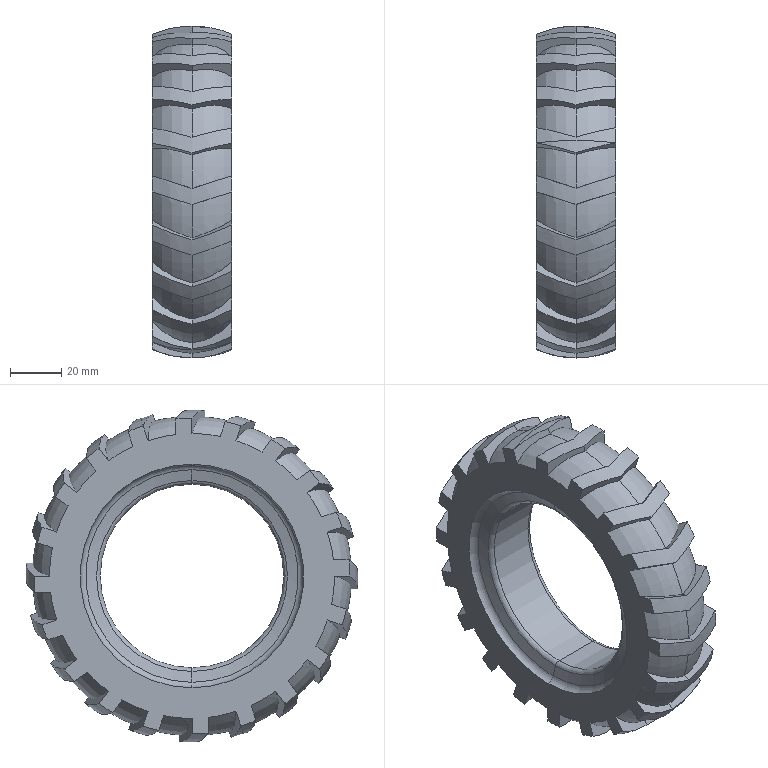Part | SolidWorks | features CirPattern 1, ICE 1, RefAxis 1, RevCut 1, Revolution 1 | 1 solid | 158 faces | box 30.833 x 129 x 129 mm | volume 226597 mm3 | plane 82 | torus 70 | cone 4 | cylinder 2 | commonest cylinder face diameters 71.352 x2